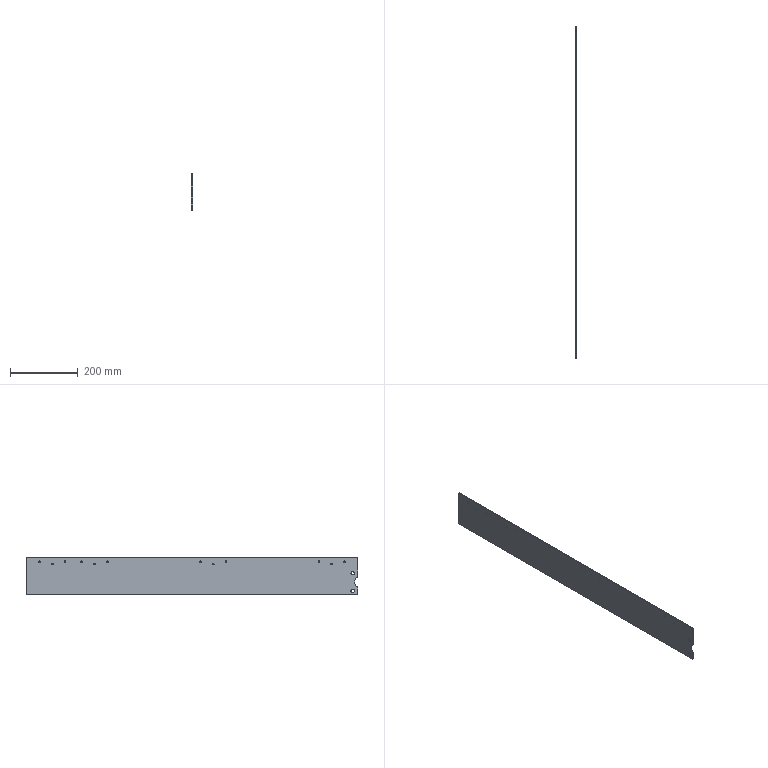Part | STEP file | HESS-408-70-15W-W-44-upper door left reinforcing plate | 1 solid | 36 faces | box 3 x 980 x 110 mm | volume 321603 mm3 | cylinder 29 | plane 7 | commonest cylinder face diameters 5 x24 10 x4 30 x1